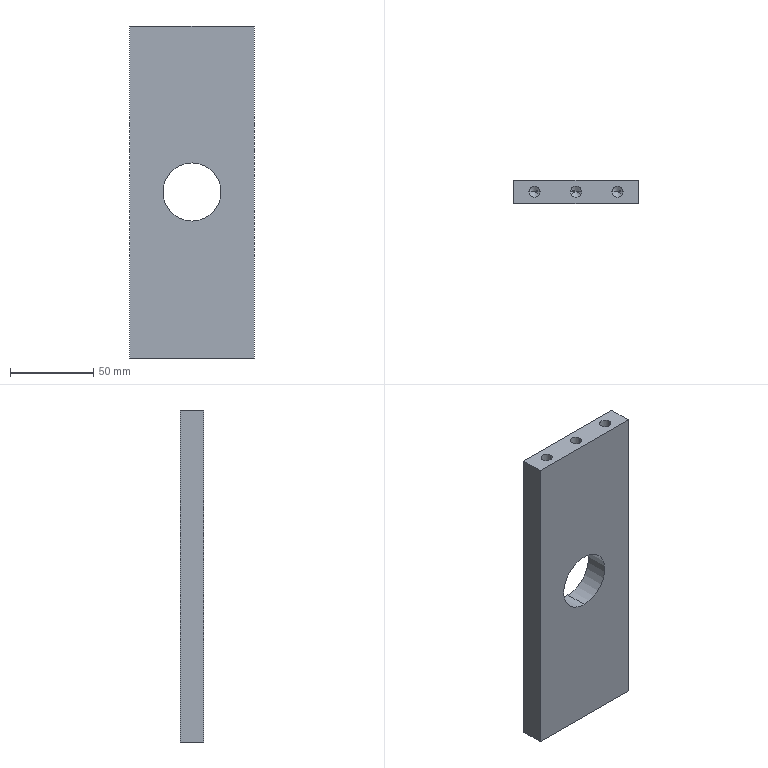Part | SolidWorks | features HoleWzd 2, Extrusion 1, ICE 1 | 1 solid | 32 faces | box 75 x 14 x 200 mm | volume 191534 mm3 | cylinder 14 | cone 12 | plane 6 | commonest cylinder face diameters 6.8 x12 35 x2
STEP:
#1=CARTESIAN_POINT('',(93.89,327.,22.25));
#2=VERTEX_POINT('',#1);
#3=CARTESIAN_POINT('',(87.09,327.,22.25));
#4=VERTEX_POINT('',#3);
#5=CARTESIAN_POINT('',(90.49,327.,22.25));
#6=DIRECTION('',(0.,0.,-1.));
#7=DIRECTION('',(-1.,0.,0.));
#8=AXIS2_PLACEMENT_3D('',#5,#6,#7);
#9=CIRCLE('',#8,3.4);
#10=EDGE_CURVE('',#2,#4,#9,.T.);
#11=ORIENTED_EDGE('',*,*,#10,.F.);
#12=CARTESIAN_POINT('',(93.89,327.,0.));
#13=VERTEX_POINT('',#12);
#14=CARTESIAN_POINT('',(93.89,327.,0.));
#15=DIRECTION('',(0.,0.,-1.));
#16=VECTOR('',#15,1000.);
#17=LINE('',#14,#16);
#18=EDGE_CURVE('',#2,#13,#17,.T.);
#19=ORIENTED_EDGE('',*,*,#18,.T.);
#20=CARTESIAN_POINT('',(87.09,327.,0.));
#21=VERTEX_POINT('',#20);
#22=CARTESIAN_POINT('',(90.49,327.,0.));
#23=DIRECTION('',(0.,0.,-1.));
#24=DIRECTION('',(-1.,0.,0.));
#25=AXIS2_PLACEMENT_3D('',#22,#23,#24);
#26=CIRCLE('',#25,3.4);
#27=EDGE_CURVE('',#13,#21,#26,.T.);
#28=ORIENTED_EDGE('',*,*,#27,.T.);
#29=CARTESIAN_POINT('',(87.09,327.,0.));
#30=DIRECTION('',(0.,0.,-1.));
#31=VECTOR('',#30,1000.);
#32=LINE('',#29,#31);
#33=EDGE_CURVE('',#4,#21,#32,.T.);
#34=ORIENTED_EDGE('',*,*,#33,.F.);
#35=EDGE_LOOP('',(#11,#19,#28,#34));
#36=FACE_OUTER_BOUND('',#35,.T.);
#37=CARTESIAN_POINT('',(90.49,327.,0.));
#38=DIRECTION('',(0.,0.,-1.));
#39=DIRECTION('',(-1.,0.,0.));
#40=AXIS2_PLACEMENT_3D('',#37,#38,#39);
#41=CYLINDRICAL_SURFACE('',#40,3.4);
#42=ADVANCED_FACE('',(#36),#41,.F.);
#43=CARTESIAN_POINT('',(90.49,327.,24.293));
#44=VERTEX_POINT('',#43);
#45=CARTESIAN_POINT('',(87.09,327.,22.25));
#46=DIRECTION('',(-0.8572,0.,-0.515));
#47=VECTOR('',#46,1000.);
#48=LINE('',#45,#47);
#49=EDGE_CURVE('',#44,#4,#48,.T.);
#50=ORIENTED_EDGE('',*,*,#49,.F.);
#51=CARTESIAN_POINT('',(93.89,327.,22.25));
#52=DIRECTION('',(0.8572,0.,-0.515));
#53=VECTOR('',#52,1000.);
#54=LINE('',#51,#53);
#55=EDGE_CURVE('',#44,#2,#54,.T.);
#56=ORIENTED_EDGE('',*,*,#55,.T.);
#57=ORIENTED_EDGE('',*,*,#10,.T.);
#58=EDGE_LOOP('',(#50,#56,#57));
#59=FACE_OUTER_BOUND('',#58,.T.);
#60=CARTESIAN_POINT('',(90.49,327.,22.25));
#61=DIRECTION('',(0.,0.,-1.));
#62=DIRECTION('',(-1.,0.,0.));
#63=AXIS2_PLACEMENT_3D('',#60,#61,#62);
#64=CONICAL_SURFACE('',#63,3.4,1.03);
#65=ADVANCED_FACE('',(#59),#64,.F.);
#66=CARTESIAN_POINT('',(68.89,327.,22.25));
#67=VERTEX_POINT('',#66);
#68=CARTESIAN_POINT('',(62.09,327.,22.25));
#69=VERTEX_POINT('',#68);
#70=CARTESIAN_POINT('',(65.49,327.,22.25));
#71=DIRECTION('',(0.,0.,-1.));
#72=DIRECTION('',(-1.,0.,0.));
#73=AXIS2_PLACEMENT_3D('',#70,#71,#72);
#74=CIRCLE('',#73,3.4);
#75=EDGE_CURVE('',#67,#69,#74,.T.);
#76=ORIENTED_EDGE('',*,*,#75,.F.);
#77=CARTESIAN_POINT('',(68.89,327.,0.));
#78=VERTEX_POINT('',#77);
#79=CARTESIAN_POINT('',(68.89,327.,0.));
#80=DIRECTION('',(0.,0.,-1.));
#81=VECTOR('',#80,1000.);
#82=LINE('',#79,#81);
#83=EDGE_CURVE('',#67,#78,#82,.T.);
#84=ORIENTED_EDGE('',*,*,#83,.T.);
#85=CARTESIAN_POINT('',(62.09,327.,0.));
#86=VERTEX_POINT('',#85);
#87=CARTESIAN_POINT('',(65.49,327.,0.));
#88=DIRECTION('',(0.,0.,-1.));
#89=DIRECTION('',(-1.,0.,0.));
#90=AXIS2_PLACEMENT_3D('',#87,#88,#89);
#91=CIRCLE('',#90,3.4);
#92=EDGE_CURVE('',#78,#86,#91,.T.);
#93=ORIENTED_EDGE('',*,*,#92,.T.);
#94=CARTESIAN_POINT('',(62.09,327.,0.));
#95=DIRECTION('',(0.,0.,-1.));
#96=VECTOR('',#95,1000.);
#97=LINE('',#94,#96);
#98=EDGE_CURVE('',#69,#86,#97,.T.);
#99=ORIENTED_EDGE('',*,*,#98,.F.);
#100=EDGE_LOOP('',(#76,#84,#93,#99));
#101=FACE_OUTER_BOUND('',#100,.T.);
#102=CARTESIAN_POINT('',(65.49,327.,0.));
#103=DIRECTION('',(0.,0.,-1.));
#104=DIRECTION('',(-1.,0.,0.));
#105=AXIS2_PLACEMENT_3D('',#102,#103,#104);
#106=CYLINDRICAL_SURFACE('',#105,3.4);
#107=ADVANCED_FACE('',(#101),#106,.F.);
#108=CARTESIAN_POINT('',(65.49,327.,24.293));
#109=VERTEX_POINT('',#108);
#110=CARTESIAN_POINT('',(62.09,327.,22.25));
#111=DIRECTION('',(-0.8572,0.,-0.515));
#112=VECTOR('',#111,1000.);
#113=LINE('',#110,#112);
#114=EDGE_CURVE('',#109,#69,#113,.T.);
#115=ORIENTED_EDGE('',*,*,#114,.F.);
#116=CARTESIAN_POINT('',(68.89,327.,22.25));
#117=DIRECTION('',(0.8572,0.,-0.515));
#118=VECTOR('',#117,1000.);
#119=LINE('',#116,#118);
#120=EDGE_CURVE('',#109,#67,#119,.T.);
#121=ORIENTED_EDGE('',*,*,#120,.T.);
#122=ORIENTED_EDGE('',*,*,#75,.T.);
#123=EDGE_LOOP('',(#115,#121,#122));
#124=FACE_OUTER_BOUND('',#123,.T.);
#125=CARTESIAN_POINT('',(65.49,327.,22.25));
#126=DIRECTION('',(0.,0.,-1.));
#127=DIRECTION('',(-1.,0.,0.));
#128=AXIS2_PLACEMENT_3D('',#125,#126,#127);
#129=CONICAL_SURFACE('',#128,3.4,1.03);
#130=ADVANCED_FACE('',(#124),#129,.F.);
#131=CARTESIAN_POINT('',(43.89,327.,22.25));
#132=VERTEX_POINT('',#131);
#133=CARTESIAN_POINT('',(37.09,327.,22.25));
#134=VERTEX_POINT('',#133);
#135=CARTESIAN_POINT('',(40.49,327.,22.25));
#136=DIRECTION('',(0.,0.,-1.));
#137=DIRECTION('',(-1.,0.,0.));
#138=AXIS2_PLACEMENT_3D('',#135,#136,#137);
#139=CIRCLE('',#138,3.4);
#140=EDGE_CURVE('',#132,#134,#139,.T.);
#141=ORIENTED_EDGE('',*,*,#140,.F.);
#142=CARTESIAN_POINT('',(43.89,327.,0.));
#143=VERTEX_POINT('',#142);
#144=CARTESIAN_POINT('',(43.89,327.,0.));
#145=DIRECTION('',(0.,0.,-1.));
#146=VECTOR('',#145,1000.);
#147=LINE('',#144,#146);
#148=EDGE_CURVE('',#132,#143,#147,.T.);
#149=ORIENTED_EDGE('',*,*,#148,.T.);
#150=CARTESIAN_POINT('',(37.09,327.,0.));
#151=VERTEX_POINT('',#150);
#152=CARTESIAN_POINT('',(40.49,327.,0.));
#153=DIRECTION('',(0.,0.,-1.));
#154=DIRECTION('',(-1.,0.,0.));
#155=AXIS2_PLACEMENT_3D('',#152,#153,#154);
#156=CIRCLE('',#155,3.4);
#157=EDGE_CURVE('',#143,#151,#156,.T.);
#158=ORIENTED_EDGE('',*,*,#157,.T.);
#159=CARTESIAN_POINT('',(37.09,327.,0.));
#160=DIRECTION('',(0.,0.,-1.));
#161=VECTOR('',#160,1000.);
#162=LINE('',#159,#161);
#163=EDGE_CURVE('',#134,#151,#162,.T.);
#164=ORIENTED_EDGE('',*,*,#163,.F.);
#165=EDGE_LOOP('',(#141,#149,#158,#164));
#166=FACE_OUTER_BOUND('',#165,.T.);
#167=CARTESIAN_POINT('',(40.49,327.,0.));
#168=DIRECTION('',(0.,0.,-1.));
#169=DIRECTION('',(-1.,0.,0.));
#170=AXIS2_PLACEMENT_3D('',#167,#168,#169);
#171=CYLINDRICAL_SURFACE('',#170,3.4);
#172=ADVANCED_FACE('',(#166),#171,.F.);
#173=CARTESIAN_POINT('',(40.49,327.,24.293));
#174=VERTEX_POINT('',#173);
#175=CARTESIAN_POINT('',(37.09,327.,22.25));
#176=DIRECTION('',(-0.8572,0.,-0.515));
#177=VECTOR('',#176,1000.);
#178=LINE('',#175,#177);
#179=EDGE_CURVE('',#174,#134,#178,.T.);
#180=ORIENTED_EDGE('',*,*,#179,.F.);
#181=CARTESIAN_POINT('',(43.89,327.,22.25));
#182=DIRECTION('',(0.8572,0.,-0.515));
#183=VECTOR('',#182,1000.);
#184=LINE('',#181,#183);
#185=EDGE_CURVE('',#174,#132,#184,.T.);
#186=ORIENTED_EDGE('',*,*,#185,.T.);
#187=ORIENTED_EDGE('',*,*,#140,.T.);
#188=EDGE_LOOP('',(#180,#186,#187));
#189=FACE_OUTER_BOUND('',#188,.T.);
#190=CARTESIAN_POINT('',(40.49,327.,22.25));
#191=DIRECTION('',(0.,0.,-1.));
#192=DIRECTION('',(-1.,0.,0.));
#193=AXIS2_PLACEMENT_3D('',#190,#191,#192);
#194=CONICAL_SURFACE('',#193,3.4,1.03);
#195=ADVANCED_FACE('',(#189),#194,.F.);
#196=CARTESIAN_POINT('',(62.09,327.,177.75));
#197=VERTEX_POINT('',#196);
#198=CARTESIAN_POINT('',(68.89,327.,177.75));
#199=VERTEX_POINT('',#198);
#200=CARTESIAN_POINT('',(65.49,327.,177.75));
#201=DIRECTION('',(0.,0.,1.));
#202=DIRECTION('',(1.,0.,0.));
#203=AXIS2_PLACEMENT_3D('',#200,#201,#202);
#204=CIRCLE('',#203,3.4);
#205=EDGE_CURVE('',#197,#199,#204,.T.);
#206=ORIENTED_EDGE('',*,*,#205,.F.);
#207=CARTESIAN_POINT('',(62.09,327.,200.));
#208=VERTEX_POINT('',#207);
#209=CARTESIAN_POINT('',(62.09,327.,200.));
#210=DIRECTION('',(0.,0.,1.));
#211=VECTOR('',#210,1000.);
#212=LINE('',#209,#211);
#213=EDGE_CURVE('',#197,#208,#212,.T.);
#214=ORIENTED_EDGE('',*,*,#213,.T.);
#215=CARTESIAN_POINT('',(68.89,327.,200.));
#216=VERTEX_POINT('',#215);
#217=CARTESIAN_POINT('',(65.49,327.,200.));
#218=DIRECTION('',(0.,0.,1.));
#219=DIRECTION('',(1.,0.,0.));
#220=AXIS2_PLACEMENT_3D('',#217,#218,#219);
#221=CIRCLE('',#220,3.4);
#222=EDGE_CURVE('',#208,#216,#221,.T.);
#223=ORIENTED_EDGE('',*,*,#222,.T.);
#224=CARTESIAN_POINT('',(68.89,327.,200.));
#225=DIRECTION('',(0.,0.,1.));
#226=VECTOR('',#225,1000.);
#227=LINE('',#224,#226);
#228=EDGE_CURVE('',#199,#216,#227,.T.);
#229=ORIENTED_EDGE('',*,*,#228,.F.);
#230=EDGE_LOOP('',(#206,#214,#223,#229));
#231=FACE_OUTER_BOUND('',#230,.T.);
#232=CARTESIAN_POINT('',(65.49,327.,200.));
#233=DIRECTION('',(0.,0.,1.));
#234=DIRECTION('',(1.,0.,0.));
#235=AXIS2_PLACEMENT_3D('',#232,#233,#234);
#236=CYLINDRICAL_SURFACE('',#235,3.4);
#237=ADVANCED_FACE('',(#231),#236,.F.);
#238=CARTESIAN_POINT('',(65.49,327.,175.707));
#239=VERTEX_POINT('',#238);
#240=CARTESIAN_POINT('',(68.89,327.,177.75));
#241=DIRECTION('',(0.8572,0.,0.515));
#242=VECTOR('',#241,1000.);
#243=LINE('',#240,#242);
#244=EDGE_CURVE('',#239,#199,#243,.T.);
#245=ORIENTED_EDGE('',*,*,#244,.F.);
#246=CARTESIAN_POINT('',(62.09,327.,177.75));
#247=DIRECTION('',(-0.8572,0.,0.515));
#248=VECTOR('',#247,1000.);
#249=LINE('',#246,#248);
#250=EDGE_CURVE('',#239,#197,#249,.T.);
#251=ORIENTED_EDGE('',*,*,#250,.T.);
#252=ORIENTED_EDGE('',*,*,#205,.T.);
#253=EDGE_LOOP('',(#245,#251,#252));
#254=FACE_OUTER_BOUND('',#253,.T.);
#255=CARTESIAN_POINT('',(65.49,327.,177.75));
#256=DIRECTION('',(0.,0.,1.));
#257=DIRECTION('',(1.,0.,0.));
#258=AXIS2_PLACEMENT_3D('',#255,#256,#257);
#259=CONICAL_SURFACE('',#258,3.4,1.03);
#260=ADVANCED_FACE('',(#254),#259,.F.);
#261=CARTESIAN_POINT('',(37.09,327.,177.75));
#262=VERTEX_POINT('',#261);
#263=CARTESIAN_POINT('',(43.89,327.,177.75));
#264=VERTEX_POINT('',#263);
#265=CARTESIAN_POINT('',(40.49,327.,177.75));
#266=DIRECTION('',(0.,0.,1.));
#267=DIRECTION('',(1.,0.,0.));
#268=AXIS2_PLACEMENT_3D('',#265,#266,#267);
#269=CIRCLE('',#268,3.4);
#270=EDGE_CURVE('',#262,#264,#269,.T.);
#271=ORIENTED_EDGE('',*,*,#270,.F.);
#272=CARTESIAN_POINT('',(37.09,327.,200.));
#273=VERTEX_POINT('',#272);
#274=CARTESIAN_POINT('',(37.09,327.,200.));
#275=DIRECTION('',(0.,0.,1.));
#276=VECTOR('',#275,1000.);
#277=LINE('',#274,#276);
#278=EDGE_CURVE('',#262,#273,#277,.T.);
#279=ORIENTED_EDGE('',*,*,#278,.T.);
#280=CARTESIAN_POINT('',(43.89,327.,200.));
#281=VERTEX_POINT('',#280);
#282=CARTESIAN_POINT('',(40.49,327.,200.));
#283=DIRECTION('',(0.,0.,1.));
#284=DIRECTION('',(1.,0.,0.));
#285=AXIS2_PLACEMENT_3D('',#282,#283,#284);
#286=CIRCLE('',#285,3.4);
#287=EDGE_CURVE('',#273,#281,#286,.T.);
#288=ORIENTED_EDGE('',*,*,#287,.T.);
#289=CARTESIAN_POINT('',(43.89,327.,200.));
#290=DIRECTION('',(0.,0.,1.));
#291=VECTOR('',#290,1000.);
#292=LINE('',#289,#291);
#293=EDGE_CURVE('',#264,#281,#292,.T.);
#294=ORIENTED_EDGE('',*,*,#293,.F.);
#295=EDGE_LOOP('',(#271,#279,#288,#294));
#296=FACE_OUTER_BOUND('',#295,.T.);
#297=CARTESIAN_POINT('',(40.49,327.,200.));
#298=DIRECTION('',(0.,0.,1.));
#299=DIRECTION('',(1.,0.,0.));
#300=AXIS2_PLACEMENT_3D('',#297,#298,#299);
#301=CYLINDRICAL_SURFACE('',#300,3.4);
#302=ADVANCED_FACE('',(#296),#301,.F.);
#303=CARTESIAN_POINT('',(40.49,327.,175.707));
#304=VERTEX_POINT('',#303);
#305=CARTESIAN_POINT('',(43.89,327.,177.75));
#306=DIRECTION('',(0.8572,0.,0.515));
#307=VECTOR('',#306,1000.);
#308=LINE('',#305,#307);
#309=EDGE_CURVE('',#304,#264,#308,.T.);
#310=ORIENTED_EDGE('',*,*,#309,.F.);
#311=CARTESIAN_POINT('',(37.09,327.,177.75));
#312=DIRECTION('',(-0.8572,0.,0.515));
#313=VECTOR('',#312,1000.);
#314=LINE('',#311,#313);
#315=EDGE_CURVE('',#304,#262,#314,.T.);
#316=ORIENTED_EDGE('',*,*,#315,.T.);
#317=ORIENTED_EDGE('',*,*,#270,.T.);
#318=EDGE_LOOP('',(#310,#316,#317));
#319=FACE_OUTER_BOUND('',#318,.T.);
#320=CARTESIAN_POINT('',(40.49,327.,177.75));
#321=DIRECTION('',(0.,0.,1.));
#322=DIRECTION('',(1.,0.,0.));
#323=AXIS2_PLACEMENT_3D('',#320,#321,#322);
#324=CONICAL_SURFACE('',#323,3.4,1.03);
#325=ADVANCED_FACE('',(#319),#324,.F.);
#326=CARTESIAN_POINT('',(87.09,327.,177.75));
#327=VERTEX_POINT('',#326);
#328=CARTESIAN_POINT('',(93.89,327.,177.75));
#329=VERTEX_POINT('',#328);
#330=CARTESIAN_POINT('',(90.49,327.,177.75));
#331=DIRECTION('',(0.,0.,1.));
#332=DIRECTION('',(1.,0.,0.));
#333=AXIS2_PLACEMENT_3D('',#330,#331,#332);
#334=CIRCLE('',#333,3.4);
#335=EDGE_CURVE('',#327,#329,#334,.T.);
#336=ORIENTED_EDGE('',*,*,#335,.F.);
#337=CARTESIAN_POINT('',(87.09,327.,200.));
#338=VERTEX_POINT('',#337);
#339=CARTESIAN_POINT('',(87.09,327.,200.));
#340=DIRECTION('',(0.,0.,1.));
#341=VECTOR('',#340,1000.);
#342=LINE('',#339,#341);
#343=EDGE_CURVE('',#327,#338,#342,.T.);
#344=ORIENTED_EDGE('',*,*,#343,.T.);
#345=CARTESIAN_POINT('',(93.89,327.,200.));
#346=VERTEX_POINT('',#345);
#347=CARTESIAN_POINT('',(90.49,327.,200.));
#348=DIRECTION('',(0.,0.,1.));
#349=DIRECTION('',(1.,0.,0.));
#350=AXIS2_PLACEMENT_3D('',#347,#348,#349);
#351=CIRCLE('',#350,3.4);
#352=EDGE_CURVE('',#338,#346,#351,.T.);
#353=ORIENTED_EDGE('',*,*,#352,.T.);
#354=CARTESIAN_POINT('',(93.89,327.,200.));
#355=DIRECTION('',(0.,0.,1.));
#356=VECTOR('',#355,1000.);
#357=LINE('',#354,#356);
#358=EDGE_CURVE('',#329,#346,#357,.T.);
#359=ORIENTED_EDGE('',*,*,#358,.F.);
#360=EDGE_LOOP('',(#336,#344,#353,#359));
#361=FACE_OUTER_BOUND('',#360,.T.);
#362=CARTESIAN_POINT('',(90.49,327.,200.));
#363=DIRECTION('',(0.,0.,1.));
#364=DIRECTION('',(1.,0.,0.));
#365=AXIS2_PLACEMENT_3D('',#362,#363,#364);
#366=CYLINDRICAL_SURFACE('',#365,3.4);
#367=ADVANCED_FACE('',(#361),#366,.F.);
#368=CARTESIAN_POINT('',(90.49,327.,175.707));
#369=VERTEX_POINT('',#368);
#370=CARTESIAN_POINT('',(93.89,327.,177.75));
#371=DIRECTION('',(0.8572,0.,0.515));
#372=VECTOR('',#371,1000.);
#373=LINE('',#370,#372);
#374=EDGE_CURVE('',#369,#329,#373,.T.);
#375=ORIENTED_EDGE('',*,*,#374,.F.);
#376=CARTESIAN_POINT('',(87.09,327.,177.75));
#377=DIRECTION('',(-0.8572,0.,0.515));
#378=VECTOR('',#377,1000.);
#379=LINE('',#376,#378);
#380=EDGE_CURVE('',#369,#327,#379,.T.);
#381=ORIENTED_EDGE('',*,*,#380,.T.);
#382=ORIENTED_EDGE('',*,*,#335,.T.);
#383=EDGE_LOOP('',(#375,#381,#382));
#384=FACE_OUTER_BOUND('',#383,.T.);
#385=CARTESIAN_POINT('',(90.49,327.,177.75));
#386=DIRECTION('',(0.,0.,1.));
#387=DIRECTION('',(1.,0.,0.));
#388=AXIS2_PLACEMENT_3D('',#385,#386,#387);
#389=CONICAL_SURFACE('',#388,3.4,1.03);
#390=ADVANCED_FACE('',(#384),#389,.F.);
#391=CARTESIAN_POINT('',(65.49,320.,82.5));
#392=VERTEX_POINT('',#391);
#393=CARTESIAN_POINT('',(65.49,320.,117.5));
#394=VERTEX_POINT('',#393);
#395=CARTESIAN_POINT('',(65.49,320.,100.));
#396=DIRECTION('',(0.,1.,0.));
#397=DIRECTION('',(0.,0.,1.));
#398=AXIS2_PLACEMENT_3D('',#395,#396,#397);
#399=CIRCLE('',#398,17.5);
#400=EDGE_CURVE('',#392,#394,#399,.T.);
#401=ORIENTED_EDGE('',*,*,#400,.F.);
#402=CARTESIAN_POINT('',(65.49,334.,82.5));
#403=VERTEX_POINT('',#402);
#404=CARTESIAN_POINT('',(65.49,320.,82.5));
#405=DIRECTION('',(0.,1.,0.));
#406=VECTOR('',#405,1000.);
#407=LINE('',#404,#406);
#408=EDGE_CURVE('',#392,#403,#407,.T.);
#409=ORIENTED_EDGE('',*,*,#408,.T.);
#410=CARTESIAN_POINT('',(65.49,334.,117.5));
#411=VERTEX_POINT('',#410);
#412=CARTESIAN_POINT('',(65.49,334.,100.));
#413=DIRECTION('',(0.,1.,0.));
#414=DIRECTION('',(0.,0.,1.));
#415=AXIS2_PLACEMENT_3D('',#412,#413,#414);
#416=CIRCLE('',#415,17.5);
#417=EDGE_CURVE('',#403,#411,#416,.T.);
#418=ORIENTED_EDGE('',*,*,#417,.T.);
#419=CARTESIAN_POINT('',(65.49,320.,117.5));
#420=DIRECTION('',(0.,1.,0.));
#421=VECTOR('',#420,1000.);
#422=LINE('',#419,#421);
#423=EDGE_CURVE('',#394,#411,#422,.T.);
#424=ORIENTED_EDGE('',*,*,#423,.F.);
#425=EDGE_LOOP('',(#401,#409,#418,#424));
#426=FACE_OUTER_BOUND('',#425,.T.);
#427=CARTESIAN_POINT('',(65.49,320.,100.));
#428=DIRECTION('',(0.,1.,0.));
#429=DIRECTION('',(0.,0.,1.));
#430=AXIS2_PLACEMENT_3D('',#427,#428,#429);
#431=CYLINDRICAL_SURFACE('',#430,17.5);
#432=ADVANCED_FACE('',(#426),#431,.F.);
#433=CARTESIAN_POINT('',(90.49,327.,0.));
#434=DIRECTION('',(0.,0.,-1.));
#435=DIRECTION('',(-1.,0.,0.));
#436=AXIS2_PLACEMENT_3D('',#433,#434,#435);
#437=CIRCLE('',#436,3.4);
#438=EDGE_CURVE('',#21,#13,#437,.T.);
#439=ORIENTED_EDGE('',*,*,#438,.F.);
#440=ORIENTED_EDGE('',*,*,#27,.F.);
#441=EDGE_LOOP('',(#439,#440));
#442=FACE_BOUND('',#441,.T.);
#443=CARTESIAN_POINT('',(65.49,327.,0.));
#444=DIRECTION('',(0.,0.,-1.));
#445=DIRECTION('',(-1.,0.,0.));
#446=AXIS2_PLACEMENT_3D('',#443,#444,#445);
#447=CIRCLE('',#446,3.4);
#448=EDGE_CURVE('',#86,#78,#447,.T.);
#449=ORIENTED_EDGE('',*,*,#448,.F.);
#450=ORIENTED_EDGE('',*,*,#92,.F.);
#451=EDGE_LOOP('',(#449,#450));
#452=FACE_BOUND('',#451,.T.);
#453=CARTESIAN_POINT('',(40.49,327.,0.));
#454=DIRECTION('',(0.,0.,-1.));
#455=DIRECTION('',(-1.,0.,0.));
#456=AXIS2_PLACEMENT_3D('',#453,#454,#455);
#457=CIRCLE('',#456,3.4);
#458=EDGE_CURVE('',#151,#143,#457,.T.);
#459=ORIENTED_EDGE('',*,*,#458,.F.);
#460=ORIENTED_EDGE('',*,*,#157,.F.);
#461=EDGE_LOOP('',(#459,#460));
#462=FACE_BOUND('',#461,.T.);
#463=CARTESIAN_POINT('',(27.99,334.,0.));
#464=VERTEX_POINT('',#463);
#465=CARTESIAN_POINT('',(27.99,320.,0.));
#466=VERTEX_POINT('',#465);
#467=CARTESIAN_POINT('',(27.99,334.,0.));
#468=DIRECTION('',(0.,-1.,0.));
#469=VECTOR('',#468,1000.);
#470=LINE('',#467,#469);
#471=EDGE_CURVE('',#464,#466,#470,.T.);
#472=ORIENTED_EDGE('',*,*,#471,.F.);
#473=CARTESIAN_POINT('',(102.99,334.,0.));
#474=VERTEX_POINT('',#473);
#475=CARTESIAN_POINT('',(27.99,334.,0.));
#476=DIRECTION('',(-1.,0.,0.));
#477=VECTOR('',#476,1000.);
#478=LINE('',#475,#477);
#479=EDGE_CURVE('',#474,#464,#478,.T.);
#480=ORIENTED_EDGE('',*,*,#479,.F.);
#481=CARTESIAN_POINT('',(102.99,320.,0.));
#482=VERTEX_POINT('',#481);
#483=CARTESIAN_POINT('',(102.99,334.,0.));
#484=DIRECTION('',(0.,1.,0.));
#485=VECTOR('',#484,1000.);
#486=LINE('',#483,#485);
#487=EDGE_CURVE('',#482,#474,#486,.T.);
#488=ORIENTED_EDGE('',*,*,#487,.F.);
#489=CARTESIAN_POINT('',(27.99,320.,0.));
#490=DIRECTION('',(1.,0.,0.));
#491=VECTOR('',#490,1000.);
#492=LINE('',#489,#491);
#493=EDGE_CURVE('',#466,#482,#492,.T.);
#494=ORIENTED_EDGE('',*,*,#493,.F.);
#495=EDGE_LOOP('',(#472,#480,#488,#494));
#496=FACE_OUTER_BOUND('',#495,.T.);
#497=CARTESIAN_POINT('',(0.,0.,0.));
#498=DIRECTION('',(0.,0.,1.));
#499=DIRECTION('',(1.,0.,0.));
#500=AXIS2_PLACEMENT_3D('',#497,#498,#499);
#501=PLANE('',#500);
#502=ADVANCED_FACE('',(#442,#452,#462,#496),#501,.F.);
#503=CARTESIAN_POINT('',(65.49,334.,100.));
#504=DIRECTION('',(0.,1.,0.));
#505=DIRECTION('',(0.,0.,1.));
#506=AXIS2_PLACEMENT_3D('',#503,#504,#505);
#507=CIRCLE('',#506,17.5);
#508=EDGE_CURVE('',#411,#403,#507,.T.);
#509=ORIENTED_EDGE('',*,*,#508,.F.);
#510=ORIENTED_EDGE('',*,*,#417,.F.);
#511=EDGE_LOOP('',(#509,#510));
#512=FACE_BOUND('',#511,.T.);
#513=CARTESIAN_POINT('',(27.99,334.,200.));
#514=VERTEX_POINT('',#513);
#515=CARTESIAN_POINT('',(27.99,334.,276.295));
#516=DIRECTION('',(0.,0.,-1.));
#517=VECTOR('',#516,1000.);
#518=LINE('',#515,#517);
#519=EDGE_CURVE('',#514,#464,#518,.T.);
#520=ORIENTED_EDGE('',*,*,#519,.F.);
#521=CARTESIAN_POINT('',(102.99,334.,200.));
#522=VERTEX_POINT('',#521);
#523=CARTESIAN_POINT('',(27.99,334.,200.));
#524=DIRECTION('',(1.,0.,0.));
#525=VECTOR('',#524,1000.);
#526=LINE('',#523,#525);
#527=EDGE_CURVE('',#514,#522,#526,.T.);
#528=ORIENTED_EDGE('',*,*,#527,.T.);
#529=CARTESIAN_POINT('',(102.99,334.,276.295));
#530=DIRECTION('',(0.,0.,-1.));
#531=VECTOR('',#530,1000.);
#532=LINE('',#529,#531);
#533=EDGE_CURVE('',#522,#474,#532,.T.);
#534=ORIENTED_EDGE('',*,*,#533,.T.);
#535=ORIENTED_EDGE('',*,*,#479,.T.);
#536=EDGE_LOOP('',(#520,#528,#534,#535));
#537=FACE_OUTER_BOUND('',#536,.T.);
#538=CARTESIAN_POINT('',(27.99,334.,276.295));
#539=DIRECTION('',(0.,-1.,0.));
#540=DIRECTION('',(0.,0.,-1.));
#541=AXIS2_PLACEMENT_3D('',#538,#539,#540);
#542=PLANE('',#541);
#543=ADVANCED_FACE('',(#512,#537),#542,.F.);
#544=ORIENTED_EDGE('',*,*,#533,.F.);
#545=CARTESIAN_POINT('',(102.99,320.,200.));
#546=VERTEX_POINT('',#545);
#547=CARTESIAN_POINT('',(102.99,334.,200.));
#548=DIRECTION('',(0.,-1.,0.));
#549=VECTOR('',#548,1000.);
#550=LINE('',#547,#549);
#551=EDGE_CURVE('',#522,#546,#550,.T.);
#552=ORIENTED_EDGE('',*,*,#551,.T.);
#553=CARTESIAN_POINT('',(102.99,320.,276.295));
#554=DIRECTION('',(0.,0.,-1.));
#555=VECTOR('',#554,1000.);
#556=LINE('',#553,#555);
#557=EDGE_CURVE('',#546,#482,#556,.T.);
#558=ORIENTED_EDGE('',*,*,#557,.T.);
#559=ORIENTED_EDGE('',*,*,#487,.T.);
#560=EDGE_LOOP('',(#544,#552,#558,#559));
#561=FACE_OUTER_BOUND('',#560,.T.);
#562=CARTESIAN_POINT('',(102.99,334.,276.295));
#563=DIRECTION('',(-1.,0.,0.));
#564=DIRECTION('',(0.,0.,1.));
#565=AXIS2_PLACEMENT_3D('',#562,#563,#564);
#566=PLANE('',#565);
#567=ADVANCED_FACE('',(#561),#566,.F.);
#568=CARTESIAN_POINT('',(65.49,320.,100.));
#569=DIRECTION('',(0.,1.,0.));
#570=DIRECTION('',(0.,0.,1.));
#571=AXIS2_PLACEMENT_3D('',#568,#569,#570);
#572=CIRCLE('',#571,17.5);
#573=EDGE_CURVE('',#394,#392,#572,.T.);
#574=ORIENTED_EDGE('',*,*,#573,.T.);
#575=ORIENTED_EDGE('',*,*,#400,.T.);
#576=EDGE_LOOP('',(#574,#575));
#577=FACE_BOUND('',#576,.T.);
#578=ORIENTED_EDGE('',*,*,#557,.F.);
#579=CARTESIAN_POINT('',(27.99,320.,200.));
#580=VERTEX_POINT('',#579);
#581=CARTESIAN_POINT('',(27.99,320.,200.));
#582=DIRECTION('',(-1.,0.,0.));
#583=VECTOR('',#582,1000.);
#584=LINE('',#581,#583);
#585=EDGE_CURVE('',#546,#580,#584,.T.);
#586=ORIENTED_EDGE('',*,*,#585,.T.);
#587=CARTESIAN_POINT('',(27.99,320.,276.295));
#588=DIRECTION('',(0.,0.,-1.));
#589=VECTOR('',#588,1000.);
#590=LINE('',#587,#589);
#591=EDGE_CURVE('',#580,#466,#590,.T.);
#592=ORIENTED_EDGE('',*,*,#591,.T.);
#593=ORIENTED_EDGE('',*,*,#493,.T.);
#594=EDGE_LOOP('',(#578,#586,#592,#593));
#595=FACE_OUTER_BOUND('',#594,.T.);
#596=CARTESIAN_POINT('',(27.99,320.,276.295));
#597=DIRECTION('',(0.,1.,0.));
#598=DIRECTION('',(0.,0.,1.));
#599=AXIS2_PLACEMENT_3D('',#596,#597,#598);
#600=PLANE('',#599);
#601=ADVANCED_FACE('',(#577,#595),#600,.F.);
#602=ORIENTED_EDGE('',*,*,#591,.F.);
#603=CARTESIAN_POINT('',(27.99,334.,200.));
#604=DIRECTION('',(0.,1.,0.));
#605=VECTOR('',#604,1000.);
#606=LINE('',#603,#605);
#607=EDGE_CURVE('',#580,#514,#606,.T.);
#608=ORIENTED_EDGE('',*,*,#607,.T.);
#609=ORIENTED_EDGE('',*,*,#519,.T.);
#610=ORIENTED_EDGE('',*,*,#471,.T.);
#611=EDGE_LOOP('',(#602,#608,#609,#610));
#612=FACE_OUTER_BOUND('',#611,.T.);
#613=CARTESIAN_POINT('',(27.99,334.,276.295));
#614=DIRECTION('',(1.,0.,0.));
#615=DIRECTION('',(0.,0.,-1.));
#616=AXIS2_PLACEMENT_3D('',#613,#614,#615);
#617=PLANE('',#616);
#618=ADVANCED_FACE('',(#612),#617,.F.);
#619=CARTESIAN_POINT('',(65.49,327.,200.));
#620=DIRECTION('',(0.,0.,1.));
#621=DIRECTION('',(1.,0.,0.));
#622=AXIS2_PLACEMENT_3D('',#619,#620,#621);
#623=CIRCLE('',#622,3.4);
#624=EDGE_CURVE('',#216,#208,#623,.T.);
#625=ORIENTED_EDGE('',*,*,#624,.F.);
#626=ORIENTED_EDGE('',*,*,#222,.F.);
#627=EDGE_LOOP('',(#625,#626));
#628=FACE_BOUND('',#627,.T.);
#629=CARTESIAN_POINT('',(40.49,327.,200.));
#630=DIRECTION('',(0.,0.,1.));
#631=DIRECTION('',(1.,0.,0.));
#632=AXIS2_PLACEMENT_3D('',#629,#630,#631);
#633=CIRCLE('',#632,3.4);
#634=EDGE_CURVE('',#281,#273,#633,.T.);
#635=ORIENTED_EDGE('',*,*,#634,.F.);
#636=ORIENTED_EDGE('',*,*,#287,.F.);
#637=EDGE_LOOP('',(#635,#636));
#638=FACE_BOUND('',#637,.T.);
#639=CARTESIAN_POINT('',(90.49,327.,200.));
#640=DIRECTION('',(0.,0.,1.));
#641=DIRECTION('',(1.,0.,0.));
#642=AXIS2_PLACEMENT_3D('',#639,#640,#641);
#643=CIRCLE('',#642,3.4);
#644=EDGE_CURVE('',#346,#338,#643,.T.);
#645=ORIENTED_EDGE('',*,*,#644,.F.);
#646=ORIENTED_EDGE('',*,*,#352,.F.);
#647=EDGE_LOOP('',(#645,#646));
#648=FACE_BOUND('',#647,.T.);
#649=ORIENTED_EDGE('',*,*,#585,.F.);
#650=ORIENTED_EDGE('',*,*,#551,.F.);
#651=ORIENTED_EDGE('',*,*,#527,.F.);
#652=ORIENTED_EDGE('',*,*,#607,.F.);
#653=EDGE_LOOP('',(#649,#650,#651,#652));
#654=FACE_OUTER_BOUND('',#653,.T.);
#655=CARTESIAN_POINT('',(110.,460.,200.));
#656=DIRECTION('',(0.,0.,-1.));
#657=DIRECTION('',(0.,1.,0.));
#658=AXIS2_PLACEMENT_3D('',#655,#656,#657);
#659=PLANE('',#658);
#660=ADVANCED_FACE('',(#628,#638,#648,#654),#659,.F.);
#661=ORIENTED_EDGE('',*,*,#408,.F.);
#662=ORIENTED_EDGE('',*,*,#573,.F.);
#663=ORIENTED_EDGE('',*,*,#423,.T.);
#664=ORIENTED_EDGE('',*,*,#508,.T.);
#665=EDGE_LOOP('',(#661,#662,#663,#664));
#666=FACE_OUTER_BOUND('',#665,.T.);
#667=CARTESIAN_POINT('',(65.49,320.,100.));
#668=DIRECTION('',(0.,1.,0.));
#669=DIRECTION('',(0.,0.,1.));
#670=AXIS2_PLACEMENT_3D('',#667,#668,#669);
#671=CYLINDRICAL_SURFACE('',#670,17.5);
#672=ADVANCED_FACE('',(#666),#671,.F.);
#673=ORIENTED_EDGE('',*,*,#380,.F.);
#674=ORIENTED_EDGE('',*,*,#374,.T.);
#675=CARTESIAN_POINT('',(90.49,327.,177.75));
#676=DIRECTION('',(0.,0.,1.));
#677=DIRECTION('',(1.,0.,0.));
#678=AXIS2_PLACEMENT_3D('',#675,#676,#677);
#679=CIRCLE('',#678,3.4);
#680=EDGE_CURVE('',#329,#327,#679,.T.);
#681=ORIENTED_EDGE('',*,*,#680,.T.);
#682=EDGE_LOOP('',(#673,#674,#681));
#683=FACE_OUTER_BOUND('',#682,.T.);
#684=CARTESIAN_POINT('',(90.49,327.,177.75));
#685=DIRECTION('',(0.,0.,1.));
#686=DIRECTION('',(1.,0.,0.));
#687=AXIS2_PLACEMENT_3D('',#684,#685,#686);
#688=CONICAL_SURFACE('',#687,3.4,1.03);
#689=ADVANCED_FACE('',(#683),#688,.F.);
#690=ORIENTED_EDGE('',*,*,#343,.F.);
#691=ORIENTED_EDGE('',*,*,#680,.F.);
#692=ORIENTED_EDGE('',*,*,#358,.T.);
#693=ORIENTED_EDGE('',*,*,#644,.T.);
#694=EDGE_LOOP('',(#690,#691,#692,#693));
#695=FACE_OUTER_BOUND('',#694,.T.);
#696=CARTESIAN_POINT('',(90.49,327.,200.));
#697=DIRECTION('',(0.,0.,1.));
#698=DIRECTION('',(1.,0.,0.));
#699=AXIS2_PLACEMENT_3D('',#696,#697,#698);
#700=CYLINDRICAL_SURFACE('',#699,3.4);
#701=ADVANCED_FACE('',(#695),#700,.F.);
#702=ORIENTED_EDGE('',*,*,#315,.F.);
#703=ORIENTED_EDGE('',*,*,#309,.T.);
#704=CARTESIAN_POINT('',(40.49,327.,177.75));
#705=DIRECTION('',(0.,0.,1.));
#706=DIRECTION('',(1.,0.,0.));
#707=AXIS2_PLACEMENT_3D('',#704,#705,#706);
#708=CIRCLE('',#707,3.4);
#709=EDGE_CURVE('',#264,#262,#708,.T.);
#710=ORIENTED_EDGE('',*,*,#709,.T.);
#711=EDGE_LOOP('',(#702,#703,#710));
#712=FACE_OUTER_BOUND('',#711,.T.);
#713=CARTESIAN_POINT('',(40.49,327.,177.75));
#714=DIRECTION('',(0.,0.,1.));
#715=DIRECTION('',(1.,0.,0.));
#716=AXIS2_PLACEMENT_3D('',#713,#714,#715);
#717=CONICAL_SURFACE('',#716,3.4,1.03);
#718=ADVANCED_FACE('',(#712),#717,.F.);
#719=ORIENTED_EDGE('',*,*,#278,.F.);
#720=ORIENTED_EDGE('',*,*,#709,.F.);
#721=ORIENTED_EDGE('',*,*,#293,.T.);
#722=ORIENTED_EDGE('',*,*,#634,.T.);
#723=EDGE_LOOP('',(#719,#720,#721,#722));
#724=FACE_OUTER_BOUND('',#723,.T.);
#725=CARTESIAN_POINT('',(40.49,327.,200.));
#726=DIRECTION('',(0.,0.,1.));
#727=DIRECTION('',(1.,0.,0.));
#728=AXIS2_PLACEMENT_3D('',#725,#726,#727);
#729=CYLINDRICAL_SURFACE('',#728,3.4);
#730=ADVANCED_FACE('',(#724),#729,.F.);
#731=ORIENTED_EDGE('',*,*,#250,.F.);
#732=ORIENTED_EDGE('',*,*,#244,.T.);
#733=CARTESIAN_POINT('',(65.49,327.,177.75));
#734=DIRECTION('',(0.,0.,1.));
#735=DIRECTION('',(1.,0.,0.));
#736=AXIS2_PLACEMENT_3D('',#733,#734,#735);
#737=CIRCLE('',#736,3.4);
#738=EDGE_CURVE('',#199,#197,#737,.T.);
#739=ORIENTED_EDGE('',*,*,#738,.T.);
#740=EDGE_LOOP('',(#731,#732,#739));
#741=FACE_OUTER_BOUND('',#740,.T.);
#742=CARTESIAN_POINT('',(65.49,327.,177.75));
#743=DIRECTION('',(0.,0.,1.));
#744=DIRECTION('',(1.,0.,0.));
#745=AXIS2_PLACEMENT_3D('',#742,#743,#744);
#746=CONICAL_SURFACE('',#745,3.4,1.03);
#747=ADVANCED_FACE('',(#741),#746,.F.);
#748=ORIENTED_EDGE('',*,*,#213,.F.);
#749=ORIENTED_EDGE('',*,*,#738,.F.);
#750=ORIENTED_EDGE('',*,*,#228,.T.);
#751=ORIENTED_EDGE('',*,*,#624,.T.);
#752=EDGE_LOOP('',(#748,#749,#750,#751));
#753=FACE_OUTER_BOUND('',#752,.T.);
#754=CARTESIAN_POINT('',(65.49,327.,200.));
#755=DIRECTION('',(0.,0.,1.));
#756=DIRECTION('',(1.,0.,0.));
#757=AXIS2_PLACEMENT_3D('',#754,#755,#756);
#758=CYLINDRICAL_SURFACE('',#757,3.4);
#759=ADVANCED_FACE('',(#753),#758,.F.);
#760=ORIENTED_EDGE('',*,*,#185,.F.);
#761=ORIENTED_EDGE('',*,*,#179,.T.);
#762=CARTESIAN_POINT('',(40.49,327.,22.25));
#763=DIRECTION('',(0.,0.,-1.));
#764=DIRECTION('',(-1.,0.,0.));
#765=AXIS2_PLACEMENT_3D('',#762,#763,#764);
#766=CIRCLE('',#765,3.4);
#767=EDGE_CURVE('',#134,#132,#766,.T.);
#768=ORIENTED_EDGE('',*,*,#767,.T.);
#769=EDGE_LOOP('',(#760,#761,#768));
#770=FACE_OUTER_BOUND('',#769,.T.);
#771=CARTESIAN_POINT('',(40.49,327.,22.25));
#772=DIRECTION('',(0.,0.,-1.));
#773=DIRECTION('',(-1.,0.,0.));
#774=AXIS2_PLACEMENT_3D('',#771,#772,#773);
#775=CONICAL_SURFACE('',#774,3.4,1.03);
#776=ADVANCED_FACE('',(#770),#775,.F.);
#777=ORIENTED_EDGE('',*,*,#148,.F.);
#778=ORIENTED_EDGE('',*,*,#767,.F.);
#779=ORIENTED_EDGE('',*,*,#163,.T.);
#780=ORIENTED_EDGE('',*,*,#458,.T.);
#781=EDGE_LOOP('',(#777,#778,#779,#780));
#782=FACE_OUTER_BOUND('',#781,.T.);
#783=CARTESIAN_POINT('',(40.49,327.,0.));
#784=DIRECTION('',(0.,0.,-1.));
#785=DIRECTION('',(-1.,0.,0.));
#786=AXIS2_PLACEMENT_3D('',#783,#784,#785);
#787=CYLINDRICAL_SURFACE('',#786,3.4);
#788=ADVANCED_FACE('',(#782),#787,.F.);
#789=ORIENTED_EDGE('',*,*,#120,.F.);
#790=ORIENTED_EDGE('',*,*,#114,.T.);
#791=CARTESIAN_POINT('',(65.49,327.,22.25));
#792=DIRECTION('',(0.,0.,-1.));
#793=DIRECTION('',(-1.,0.,0.));
#794=AXIS2_PLACEMENT_3D('',#791,#792,#793);
#795=CIRCLE('',#794,3.4);
#796=EDGE_CURVE('',#69,#67,#795,.T.);
#797=ORIENTED_EDGE('',*,*,#796,.T.);
#798=EDGE_LOOP('',(#789,#790,#797));
#799=FACE_OUTER_BOUND('',#798,.T.);
#800=CARTESIAN_POINT('',(65.49,327.,22.25));
#801=DIRECTION('',(0.,0.,-1.));
#802=DIRECTION('',(-1.,0.,0.));
#803=AXIS2_PLACEMENT_3D('',#800,#801,#802);
#804=CONICAL_SURFACE('',#803,3.4,1.03);
#805=ADVANCED_FACE('',(#799),#804,.F.);
#806=ORIENTED_EDGE('',*,*,#83,.F.);
#807=ORIENTED_EDGE('',*,*,#796,.F.);
#808=ORIENTED_EDGE('',*,*,#98,.T.);
#809=ORIENTED_EDGE('',*,*,#448,.T.);
#810=EDGE_LOOP('',(#806,#807,#808,#809));
#811=FACE_OUTER_BOUND('',#810,.T.);
#812=CARTESIAN_POINT('',(65.49,327.,0.));
#813=DIRECTION('',(0.,0.,-1.));
#814=DIRECTION('',(-1.,0.,0.));
#815=AXIS2_PLACEMENT_3D('',#812,#813,#814);
#816=CYLINDRICAL_SURFACE('',#815,3.4);
#817=ADVANCED_FACE('',(#811),#816,.F.);
#818=ORIENTED_EDGE('',*,*,#55,.F.);
#819=ORIENTED_EDGE('',*,*,#49,.T.);
#820=CARTESIAN_POINT('',(90.49,327.,22.25));
#821=DIRECTION('',(0.,0.,-1.));
#822=DIRECTION('',(-1.,0.,0.));
#823=AXIS2_PLACEMENT_3D('',#820,#821,#822);
#824=CIRCLE('',#823,3.4);
#825=EDGE_CURVE('',#4,#2,#824,.T.);
#826=ORIENTED_EDGE('',*,*,#825,.T.);
#827=EDGE_LOOP('',(#818,#819,#826));
#828=FACE_OUTER_BOUND('',#827,.T.);
#829=CARTESIAN_POINT('',(90.49,327.,22.25));
#830=DIRECTION('',(0.,0.,-1.));
#831=DIRECTION('',(-1.,0.,0.));
#832=AXIS2_PLACEMENT_3D('',#829,#830,#831);
#833=CONICAL_SURFACE('',#832,3.4,1.03);
#834=ADVANCED_FACE('',(#828),#833,.F.);
#835=ORIENTED_EDGE('',*,*,#18,.F.);
#836=ORIENTED_EDGE('',*,*,#825,.F.);
#837=ORIENTED_EDGE('',*,*,#33,.T.);
#838=ORIENTED_EDGE('',*,*,#438,.T.);
#839=EDGE_LOOP('',(#835,#836,#837,#838));
#840=FACE_OUTER_BOUND('',#839,.T.);
#841=CARTESIAN_POINT('',(90.49,327.,0.));
#842=DIRECTION('',(0.,0.,-1.));
#843=DIRECTION('',(-1.,0.,0.));
#844=AXIS2_PLACEMENT_3D('',#841,#842,#843);
#845=CYLINDRICAL_SURFACE('',#844,3.4);
#846=ADVANCED_FACE('',(#840),#845,.F.);
#847=CLOSED_SHELL('',(#42,#65,#107,#130,#172,#195,#237,#260,#302,#325,#367,#390,#432,#502,#543,#567,#601,#618,#660,#672,#689,#701,#718,#730,#747,#759,#776,#788,#805,#817,#834,#846));
#848=MANIFOLD_SOLID_BREP('',#847);
#849=CARTESIAN_POINT('',(0.,0.,0.));
#850=DIRECTION('',(0.,0.,1.));
#851=DIRECTION('',(1.,0.,0.));
#852=AXIS2_PLACEMENT_3D('',#849,#850,#851);
#853=(LENGTH_UNIT()NAMED_UNIT(*)SI_UNIT(.MILLI.,.METRE.));
#854=UNCERTAINTY_MEASURE_WITH_UNIT(LENGTH_MEASURE(0.00001),#853,'','');
#855=(NAMED_UNIT(*)PLANE_ANGLE_UNIT()SI_UNIT($,.RADIAN.));
#856=(NAMED_UNIT(*)SI_UNIT($,.STERADIAN.)SOLID_ANGLE_UNIT());
#857=(GEOMETRIC_REPRESENTATION_CONTEXT(3)GLOBAL_UNCERTAINTY_ASSIGNED_CONTEXT((#854))GLOBAL_UNIT_ASSIGNED_CONTEXT((#853,#855,#856))REPRESENTATION_CONTEXT('',''));
#858=ADVANCED_BREP_SHAPE_REPRESENTATION('',(#848,#852),#857);